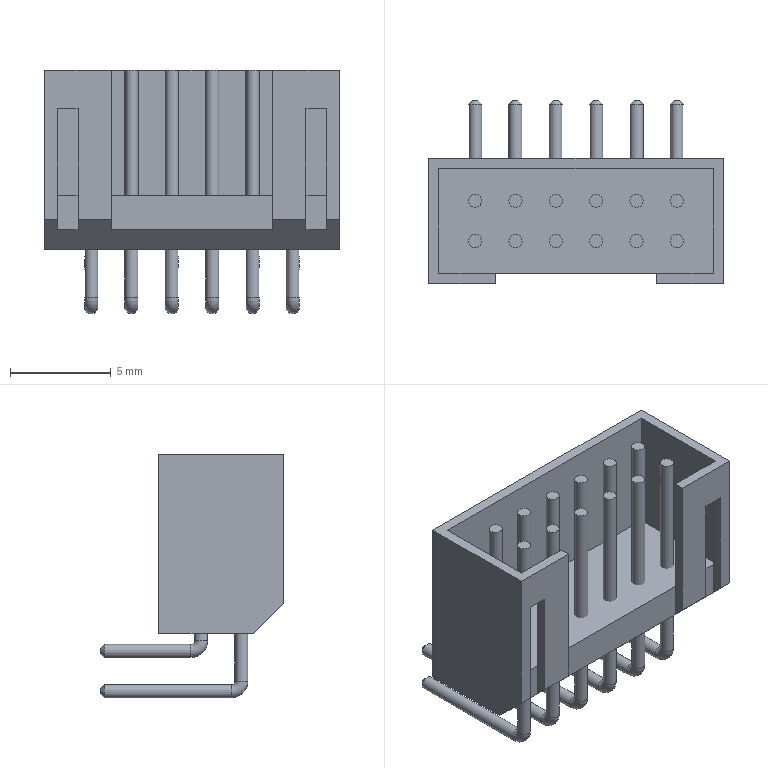Part | STEP file | JL24-12ZJW | 25 solids | 133 faces | box 14.6 x 9.1 x 12.075 mm | volume 379.843 mm3 | plane 73 | cylinder 36 | torus 12 | cone 12 | commonest cylinder face diameters 0.65 x36